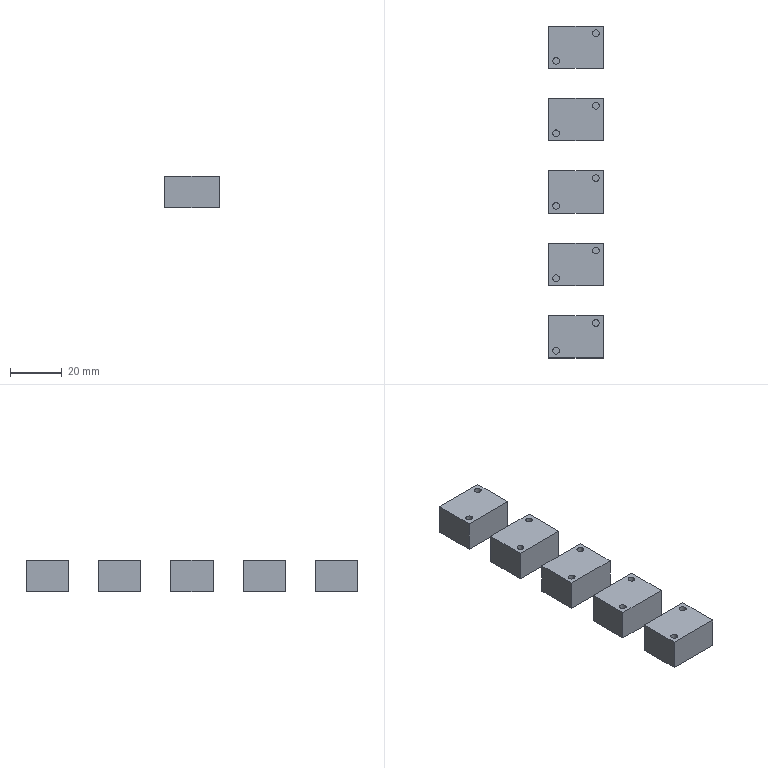NC program | NX | posted with a generic post | part box 21 x 128.262 x 12 mm
Lines 1 to 58 of 3295:
N10 G17 G21 G94 G90
(FLOOR_WALL , TOOL : D63)
N12 T01 M6
N14 G54
N16 G17 G0 G90 X100.631 Y0. S6500 M3
N18 G43 Z30. H1
N20 Z3.
N22 G94 G1 Z0. F1250.
N24 X97.631
N26 X-97.631
N28 X-100.631
N30 Z3.
N32 G0 Z30.
N34 M5
(DRILLING , TOOL : D6A45)
N36 T07 M6
N38 G54
N40 G17 G0 G90 X-61.331 Y7.7 S5000 M3
N42 G43 Z30. H7
N44 G94 G81 G98 Z-1.4 F250. R3.
N46 X-50.669 Y-7.7
N48 X-33.331 Y7.7
N50 X-22.669 Y-7.7
N52 X-5.331 Y7.7
N54 X5.331 Y-7.7
N56 X22.669 Y7.7
N58 X33.331 Y-7.7
N60 X50.669 Y7.7
N62 X61.331 Y-7.7
N64 G80
N66 G0 X61.331 Y-7.7 Z30.
N68 M5
(DRILLING_COPY , TOOL : 2.6ZT)
N70 T12 M6
N72 G54
N74 G17 G0 G90 X-61.331 Y7.7 S2000 M3
N76 G43 Z30. H12
N78 G94 G83 G98 Z-8.781 F120. Q2. R3.
N80 X-50.669 Y-7.7
N82 X-33.331 Y7.7
N84 X-22.669 Y-7.7
N86 X-5.331 Y7.7
N88 X5.331 Y-7.7
N90 X22.669 Y7.7
N92 X33.331 Y-7.7
N94 X50.669 Y7.7
N96 X61.331 Y-7.7
N98 G80
N100 G0 X61.331 Y-7.7 Z30.
N102 M5